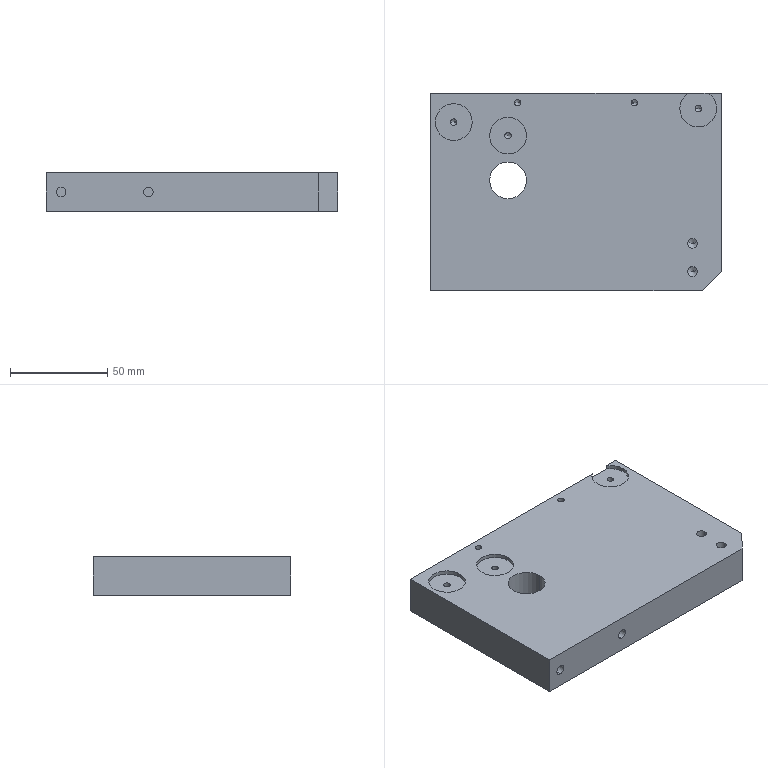Part | STEP file | Front rail (left) | 1 solid | 74 faces | box 150 x 102 x 20 mm | volume 295247 mm3 | cylinder 39 | cone 20 | plane 15 | commonest cylinder face diameters 3.3 x10 19 x9 5 x8 4 x6 4.2 x6